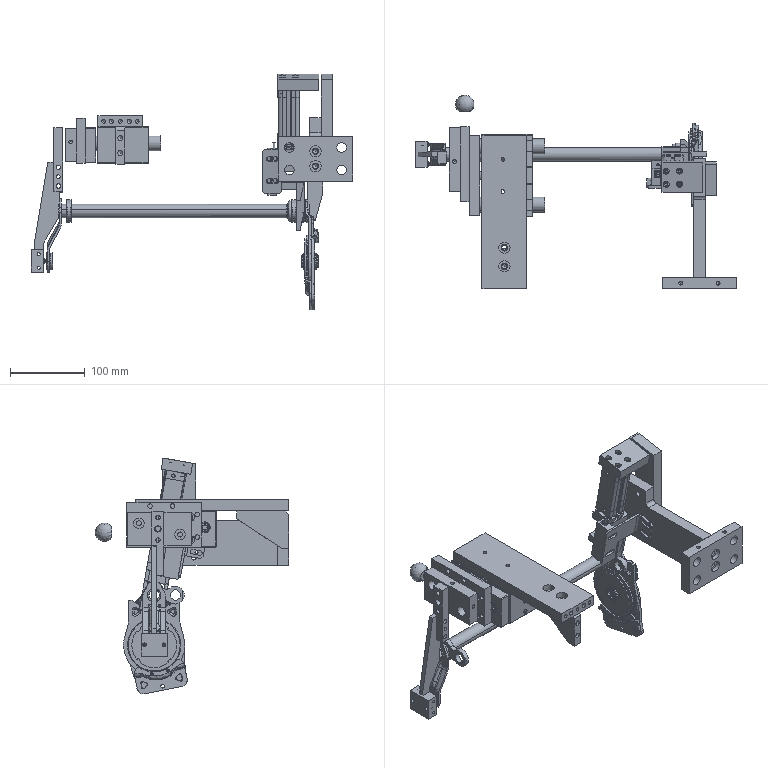Part | NX | features BREP 44 | 49 solids | 3564 faces | volume 1377004 mm3 | cylinder 1346 | plane 1232 | spline 436 | cone 289 | torus 224 | sphere 37 | commonest cylinder face diameters 0.3 x169 0.6 x144 6 x65 1 x58 3 x47 0.8 x46